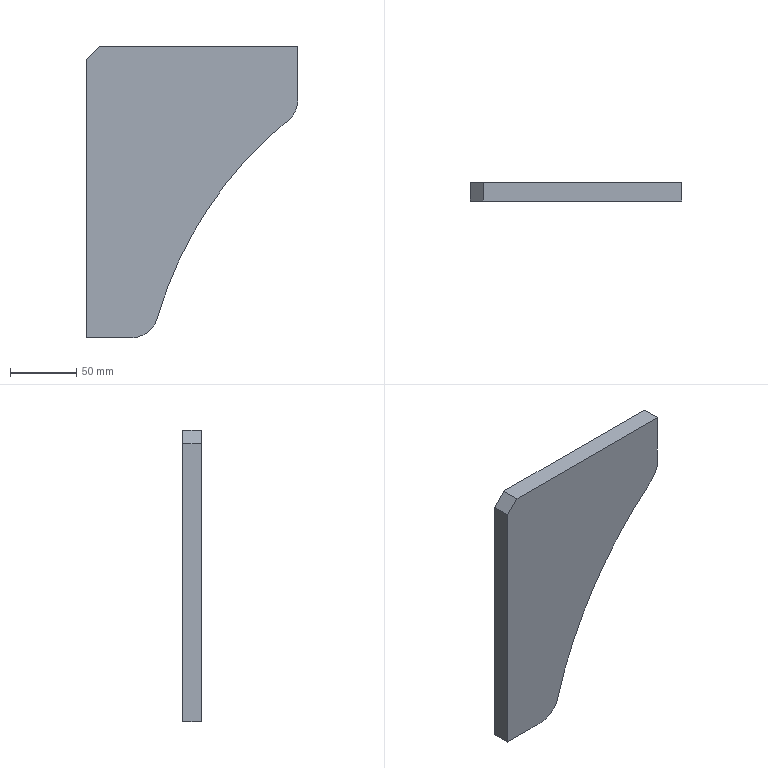Part | SolidWorks | features BaseBody 1 | 1 solid | 10 faces | box 160 x 14 x 220 mm | volume 326927 mm3 | plane 7 | cylinder 3 | commonest cylinder face diameters 40 x2 600 x1
STEP:
#1=CARTESIAN_POINT('',(-80.,-7.,-110.));
#2=VERTEX_POINT('',#1);
#3=CARTESIAN_POINT('',(-80.,-7.,100.));
#4=VERTEX_POINT('',#3);
#5=CARTESIAN_POINT('',(-80.,-7.,-110.));
#6=DIRECTION('',(0.,0.,1.));
#7=VECTOR('',#6,1000.);
#8=LINE('',#5,#7);
#9=EDGE_CURVE('',#2,#4,#8,.T.);
#10=ORIENTED_EDGE('',*,*,#9,.T.);
#11=CARTESIAN_POINT('',(-80.,7.,100.));
#12=VERTEX_POINT('',#11);
#13=CARTESIAN_POINT('',(-80.,7.,100.));
#14=DIRECTION('',(0.,-1.,0.));
#15=VECTOR('',#14,1000.);
#16=LINE('',#13,#15);
#17=EDGE_CURVE('',#12,#4,#16,.T.);
#18=ORIENTED_EDGE('',*,*,#17,.F.);
#19=CARTESIAN_POINT('',(-80.,7.,-110.));
#20=VERTEX_POINT('',#19);
#21=CARTESIAN_POINT('',(-80.,7.,-110.));
#22=DIRECTION('',(0.,0.,1.));
#23=VECTOR('',#22,1000.);
#24=LINE('',#21,#23);
#25=EDGE_CURVE('',#20,#12,#24,.T.);
#26=ORIENTED_EDGE('',*,*,#25,.F.);
#27=CARTESIAN_POINT('',(-80.,7.,-110.));
#28=DIRECTION('',(0.,-1.,0.));
#29=VECTOR('',#28,1000.);
#30=LINE('',#27,#29);
#31=EDGE_CURVE('',#20,#2,#30,.T.);
#32=ORIENTED_EDGE('',*,*,#31,.T.);
#33=EDGE_LOOP('',(#10,#18,#26,#32));
#34=FACE_OUTER_BOUND('',#33,.T.);
#35=CARTESIAN_POINT('',(-80.,7.,-110.));
#36=DIRECTION('',(1.,0.,0.));
#37=DIRECTION('',(0.,0.,-1.));
#38=AXIS2_PLACEMENT_3D('',#35,#36,#37);
#39=PLANE('',#38);
#40=ADVANCED_FACE('',(#34),#39,.F.);
#41=CARTESIAN_POINT('',(-70.,-7.,110.));
#42=VERTEX_POINT('',#41);
#43=CARTESIAN_POINT('',(-80.,-7.,100.));
#44=DIRECTION('',(0.7071,0.,0.7071));
#45=VECTOR('',#44,1000.);
#46=LINE('',#43,#45);
#47=EDGE_CURVE('',#4,#42,#46,.T.);
#48=ORIENTED_EDGE('',*,*,#47,.T.);
#49=CARTESIAN_POINT('',(-70.,7.,110.));
#50=VERTEX_POINT('',#49);
#51=CARTESIAN_POINT('',(-70.,7.,110.));
#52=DIRECTION('',(0.,-1.,0.));
#53=VECTOR('',#52,1000.);
#54=LINE('',#51,#53);
#55=EDGE_CURVE('',#50,#42,#54,.T.);
#56=ORIENTED_EDGE('',*,*,#55,.F.);
#57=CARTESIAN_POINT('',(-80.,7.,100.));
#58=DIRECTION('',(0.7071,0.,0.7071));
#59=VECTOR('',#58,1000.);
#60=LINE('',#57,#59);
#61=EDGE_CURVE('',#12,#50,#60,.T.);
#62=ORIENTED_EDGE('',*,*,#61,.F.);
#63=ORIENTED_EDGE('',*,*,#17,.T.);
#64=EDGE_LOOP('',(#48,#56,#62,#63));
#65=FACE_OUTER_BOUND('',#64,.T.);
#66=CARTESIAN_POINT('',(-80.,7.,100.));
#67=DIRECTION('',(0.7071,0.,-0.7071));
#68=DIRECTION('',(-0.7071,0.,-0.7071));
#69=AXIS2_PLACEMENT_3D('',#66,#67,#68);
#70=PLANE('',#69);
#71=ADVANCED_FACE('',(#65),#70,.F.);
#72=CARTESIAN_POINT('',(80.,-7.,110.));
#73=VERTEX_POINT('',#72);
#74=CARTESIAN_POINT('',(-70.,-7.,110.));
#75=DIRECTION('',(1.,0.,0.));
#76=VECTOR('',#75,1000.);
#77=LINE('',#74,#76);
#78=EDGE_CURVE('',#42,#73,#77,.T.);
#79=ORIENTED_EDGE('',*,*,#78,.T.);
#80=CARTESIAN_POINT('',(80.,7.,110.));
#81=VERTEX_POINT('',#80);
#82=CARTESIAN_POINT('',(80.,7.,110.));
#83=DIRECTION('',(0.,-1.,0.));
#84=VECTOR('',#83,1000.);
#85=LINE('',#82,#84);
#86=EDGE_CURVE('',#81,#73,#85,.T.);
#87=ORIENTED_EDGE('',*,*,#86,.F.);
#88=CARTESIAN_POINT('',(-70.,7.,110.));
#89=DIRECTION('',(1.,0.,0.));
#90=VECTOR('',#89,1000.);
#91=LINE('',#88,#90);
#92=EDGE_CURVE('',#50,#81,#91,.T.);
#93=ORIENTED_EDGE('',*,*,#92,.F.);
#94=ORIENTED_EDGE('',*,*,#55,.T.);
#95=EDGE_LOOP('',(#79,#87,#93,#94));
#96=FACE_OUTER_BOUND('',#95,.T.);
#97=CARTESIAN_POINT('',(-70.,7.,110.));
#98=DIRECTION('',(0.,0.,-1.));
#99=DIRECTION('',(-1.,0.,0.));
#100=AXIS2_PLACEMENT_3D('',#97,#98,#99);
#101=PLANE('',#100);
#102=ADVANCED_FACE('',(#96),#101,.F.);
#103=CARTESIAN_POINT('',(80.,-7.,69.694));
#104=VERTEX_POINT('',#103);
#105=CARTESIAN_POINT('',(80.,-7.,110.));
#106=DIRECTION('',(0.,0.,-1.));
#107=VECTOR('',#106,1000.);
#108=LINE('',#105,#107);
#109=EDGE_CURVE('',#73,#104,#108,.T.);
#110=ORIENTED_EDGE('',*,*,#109,.T.);
#111=CARTESIAN_POINT('',(80.,7.,69.694));
#112=VERTEX_POINT('',#111);
#113=CARTESIAN_POINT('',(80.,7.,69.694));
#114=DIRECTION('',(0.,-1.,0.));
#115=VECTOR('',#114,1000.);
#116=LINE('',#113,#115);
#117=EDGE_CURVE('',#112,#104,#116,.T.);
#118=ORIENTED_EDGE('',*,*,#117,.F.);
#119=CARTESIAN_POINT('',(80.,7.,110.));
#120=DIRECTION('',(0.,0.,-1.));
#121=VECTOR('',#120,1000.);
#122=LINE('',#119,#121);
#123=EDGE_CURVE('',#81,#112,#122,.T.);
#124=ORIENTED_EDGE('',*,*,#123,.F.);
#125=ORIENTED_EDGE('',*,*,#86,.T.);
#126=EDGE_LOOP('',(#110,#118,#124,#125));
#127=FACE_OUTER_BOUND('',#126,.T.);
#128=CARTESIAN_POINT('',(80.,7.,110.));
#129=DIRECTION('',(-1.,0.,0.));
#130=DIRECTION('',(0.,0.,1.));
#131=AXIS2_PLACEMENT_3D('',#128,#129,#130);
#132=PLANE('',#131);
#133=ADVANCED_FACE('',(#127),#132,.F.);
#134=CARTESIAN_POINT('',(72.631,-7.,54.187));
#135=VERTEX_POINT('',#134);
#136=CARTESIAN_POINT('',(60.,-7.,69.694));
#137=DIRECTION('',(0.,1.,0.));
#138=DIRECTION('',(0.,0.,1.));
#139=AXIS2_PLACEMENT_3D('',#136,#137,#138);
#140=CIRCLE('',#139,20.);
#141=EDGE_CURVE('',#104,#135,#140,.T.);
#142=ORIENTED_EDGE('',*,*,#141,.T.);
#143=CARTESIAN_POINT('',(72.631,7.,54.187));
#144=VERTEX_POINT('',#143);
#145=CARTESIAN_POINT('',(72.631,7.,54.187));
#146=DIRECTION('',(0.,-1.,0.));
#147=VECTOR('',#146,1000.);
#148=LINE('',#145,#147);
#149=EDGE_CURVE('',#144,#135,#148,.T.);
#150=ORIENTED_EDGE('',*,*,#149,.F.);
#151=CARTESIAN_POINT('',(60.,7.,69.694));
#152=DIRECTION('',(0.,1.,0.));
#153=DIRECTION('',(0.,0.,1.));
#154=AXIS2_PLACEMENT_3D('',#151,#152,#153);
#155=CIRCLE('',#154,20.);
#156=EDGE_CURVE('',#112,#144,#155,.T.);
#157=ORIENTED_EDGE('',*,*,#156,.F.);
#158=ORIENTED_EDGE('',*,*,#117,.T.);
#159=EDGE_LOOP('',(#142,#150,#157,#158));
#160=FACE_OUTER_BOUND('',#159,.T.);
#161=CARTESIAN_POINT('',(60.,7.,69.694));
#162=DIRECTION('',(0.,-1.,0.));
#163=DIRECTION('',(0.,0.,-1.));
#164=AXIS2_PLACEMENT_3D('',#161,#162,#163);
#165=CYLINDRICAL_SURFACE('',#164,20.);
#166=ADVANCED_FACE('',(#160),#165,.T.);
#167=CARTESIAN_POINT('',(-26.227,-7.,-95.526));
#168=VERTEX_POINT('',#167);
#169=CARTESIAN_POINT('',(262.095,-7.,-178.414));
#170=DIRECTION('',(0.,-1.,0.));
#171=DIRECTION('',(0.,0.,1.));
#172=AXIS2_PLACEMENT_3D('',#169,#170,#171);
#173=CIRCLE('',#172,300.);
#174=EDGE_CURVE('',#135,#168,#173,.T.);
#175=ORIENTED_EDGE('',*,*,#174,.T.);
#176=CARTESIAN_POINT('',(-26.227,7.,-95.526));
#177=VERTEX_POINT('',#176);
#178=CARTESIAN_POINT('',(-26.227,7.,-95.526));
#179=DIRECTION('',(0.,-1.,0.));
#180=VECTOR('',#179,1000.);
#181=LINE('',#178,#180);
#182=EDGE_CURVE('',#177,#168,#181,.T.);
#183=ORIENTED_EDGE('',*,*,#182,.F.);
#184=CARTESIAN_POINT('',(262.095,7.,-178.414));
#185=DIRECTION('',(0.,-1.,0.));
#186=DIRECTION('',(0.,0.,1.));
#187=AXIS2_PLACEMENT_3D('',#184,#185,#186);
#188=CIRCLE('',#187,300.);
#189=EDGE_CURVE('',#144,#177,#188,.T.);
#190=ORIENTED_EDGE('',*,*,#189,.F.);
#191=ORIENTED_EDGE('',*,*,#149,.T.);
#192=EDGE_LOOP('',(#175,#183,#190,#191));
#193=FACE_OUTER_BOUND('',#192,.T.);
#194=CARTESIAN_POINT('',(262.095,7.,-178.414));
#195=DIRECTION('',(0.,-1.,0.));
#196=DIRECTION('',(0.,0.,-1.));
#197=AXIS2_PLACEMENT_3D('',#194,#195,#196);
#198=CYLINDRICAL_SURFACE('',#197,300.);
#199=ADVANCED_FACE('',(#193),#198,.F.);
#200=CARTESIAN_POINT('',(-45.448,-7.,-110.));
#201=VERTEX_POINT('',#200);
#202=CARTESIAN_POINT('',(-45.448,-7.,-90.));
#203=DIRECTION('',(0.,1.,0.));
#204=DIRECTION('',(0.,0.,-1.));
#205=AXIS2_PLACEMENT_3D('',#202,#203,#204);
#206=CIRCLE('',#205,20.);
#207=EDGE_CURVE('',#168,#201,#206,.T.);
#208=ORIENTED_EDGE('',*,*,#207,.T.);
#209=CARTESIAN_POINT('',(-45.448,7.,-110.));
#210=VERTEX_POINT('',#209);
#211=CARTESIAN_POINT('',(-45.448,7.,-110.));
#212=DIRECTION('',(0.,-1.,0.));
#213=VECTOR('',#212,1000.);
#214=LINE('',#211,#213);
#215=EDGE_CURVE('',#210,#201,#214,.T.);
#216=ORIENTED_EDGE('',*,*,#215,.F.);
#217=CARTESIAN_POINT('',(-45.448,7.,-90.));
#218=DIRECTION('',(0.,1.,0.));
#219=DIRECTION('',(0.,0.,-1.));
#220=AXIS2_PLACEMENT_3D('',#217,#218,#219);
#221=CIRCLE('',#220,20.);
#222=EDGE_CURVE('',#177,#210,#221,.T.);
#223=ORIENTED_EDGE('',*,*,#222,.F.);
#224=ORIENTED_EDGE('',*,*,#182,.T.);
#225=EDGE_LOOP('',(#208,#216,#223,#224));
#226=FACE_OUTER_BOUND('',#225,.T.);
#227=CARTESIAN_POINT('',(-45.448,7.,-90.));
#228=DIRECTION('',(0.,-1.,0.));
#229=DIRECTION('',(0.,0.,-1.));
#230=AXIS2_PLACEMENT_3D('',#227,#228,#229);
#231=CYLINDRICAL_SURFACE('',#230,20.);
#232=ADVANCED_FACE('',(#226),#231,.T.);
#233=CARTESIAN_POINT('',(-45.448,-7.,-110.));
#234=DIRECTION('',(-1.,0.,0.));
#235=VECTOR('',#234,1000.);
#236=LINE('',#233,#235);
#237=EDGE_CURVE('',#201,#2,#236,.T.);
#238=ORIENTED_EDGE('',*,*,#237,.T.);
#239=ORIENTED_EDGE('',*,*,#31,.F.);
#240=CARTESIAN_POINT('',(-45.448,7.,-110.));
#241=DIRECTION('',(-1.,0.,0.));
#242=VECTOR('',#241,1000.);
#243=LINE('',#240,#242);
#244=EDGE_CURVE('',#210,#20,#243,.T.);
#245=ORIENTED_EDGE('',*,*,#244,.F.);
#246=ORIENTED_EDGE('',*,*,#215,.T.);
#247=EDGE_LOOP('',(#238,#239,#245,#246));
#248=FACE_OUTER_BOUND('',#247,.T.);
#249=CARTESIAN_POINT('',(-45.448,7.,-110.));
#250=DIRECTION('',(0.,0.,1.));
#251=DIRECTION('',(1.,0.,0.));
#252=AXIS2_PLACEMENT_3D('',#249,#250,#251);
#253=PLANE('',#252);
#254=ADVANCED_FACE('',(#248),#253,.F.);
#255=ORIENTED_EDGE('',*,*,#25,.T.);
#256=ORIENTED_EDGE('',*,*,#61,.T.);
#257=ORIENTED_EDGE('',*,*,#92,.T.);
#258=ORIENTED_EDGE('',*,*,#123,.T.);
#259=ORIENTED_EDGE('',*,*,#156,.T.);
#260=ORIENTED_EDGE('',*,*,#189,.T.);
#261=ORIENTED_EDGE('',*,*,#222,.T.);
#262=ORIENTED_EDGE('',*,*,#244,.T.);
#263=EDGE_LOOP('',(#255,#256,#257,#258,#259,#260,#261,#262));
#264=FACE_OUTER_BOUND('',#263,.T.);
#265=CARTESIAN_POINT('',(60.,7.,69.694));
#266=DIRECTION('',(0.,1.,0.));
#267=DIRECTION('',(0.,0.,1.));
#268=AXIS2_PLACEMENT_3D('',#265,#266,#267);
#269=PLANE('',#268);
#270=ADVANCED_FACE('',(#264),#269,.T.);
#271=ORIENTED_EDGE('',*,*,#9,.F.);
#272=ORIENTED_EDGE('',*,*,#237,.F.);
#273=ORIENTED_EDGE('',*,*,#207,.F.);
#274=ORIENTED_EDGE('',*,*,#174,.F.);
#275=ORIENTED_EDGE('',*,*,#141,.F.);
#276=ORIENTED_EDGE('',*,*,#109,.F.);
#277=ORIENTED_EDGE('',*,*,#78,.F.);
#278=ORIENTED_EDGE('',*,*,#47,.F.);
#279=EDGE_LOOP('',(#271,#272,#273,#274,#275,#276,#277,#278));
#280=FACE_OUTER_BOUND('',#279,.T.);
#281=CARTESIAN_POINT('',(60.,-7.,69.694));
#282=DIRECTION('',(0.,1.,0.));
#283=DIRECTION('',(0.,0.,1.));
#284=AXIS2_PLACEMENT_3D('',#281,#282,#283);
#285=PLANE('',#284);
#286=ADVANCED_FACE('',(#280),#285,.F.);
#287=CLOSED_SHELL('',(#40,#71,#102,#133,#166,#199,#232,#254,#270,#286));
#288=MANIFOLD_SOLID_BREP('',#287);
#289=CARTESIAN_POINT('',(0.,0.,0.));
#290=DIRECTION('',(0.,0.,1.));
#291=DIRECTION('',(1.,0.,0.));
#292=AXIS2_PLACEMENT_3D('',#289,#290,#291);
#293=(LENGTH_UNIT()NAMED_UNIT(*)SI_UNIT(.MILLI.,.METRE.));
#294=UNCERTAINTY_MEASURE_WITH_UNIT(LENGTH_MEASURE(0.00001),#293,'','');
#295=(NAMED_UNIT(*)PLANE_ANGLE_UNIT()SI_UNIT($,.RADIAN.));
#296=(NAMED_UNIT(*)SI_UNIT($,.STERADIAN.)SOLID_ANGLE_UNIT());
#297=(GEOMETRIC_REPRESENTATION_CONTEXT(3)GLOBAL_UNCERTAINTY_ASSIGNED_CONTEXT((#294))GLOBAL_UNIT_ASSIGNED_CONTEXT((#293,#295,#296))REPRESENTATION_CONTEXT('',''));
#298=ADVANCED_BREP_SHAPE_REPRESENTATION('',(#288,#292),#297);